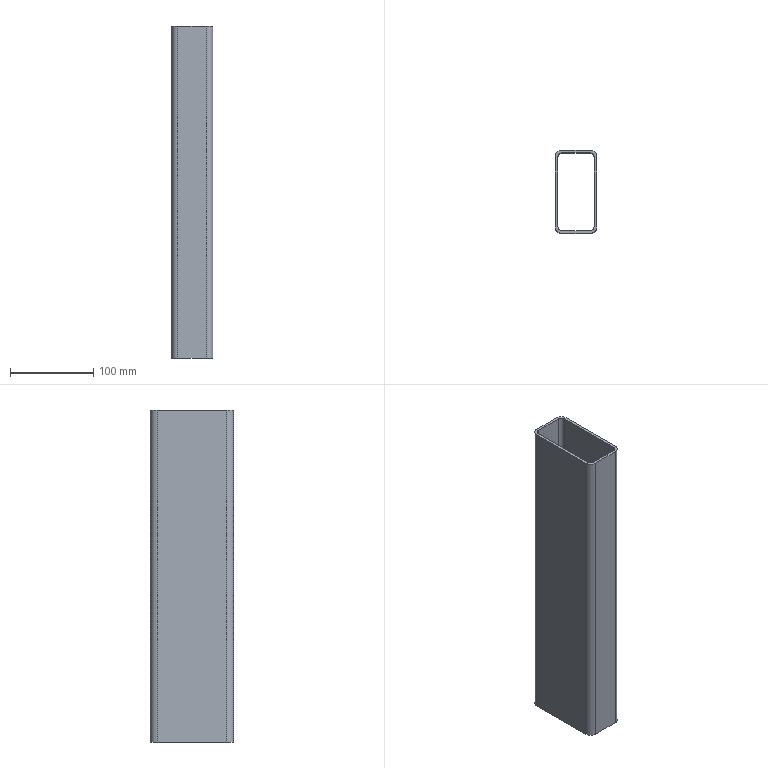Part | STEP file | KS D 3568 - 100 x 50 x 3.2 - 400 | 1 solid | 18 faces | box 50 x 100 x 400 mm | volume 353552 mm3 | plane 10 | cylinder 8 | commonest cylinder face diameters 9.6 x4 16 x4
STEP:
#1=CARTESIAN_POINT('',(0.,0.,0.));
#2=DIRECTION('',(0.,0.,1.));
#3=DIRECTION('',(1.,0.,0.));
#4=AXIS2_PLACEMENT_3D('',#1,#2,#3);
#5=CARTESIAN_POINT('',(17.,46.8,500.));
#6=VERTEX_POINT('',#5);
#7=CARTESIAN_POINT('',(-17.,46.8,500.));
#8=VERTEX_POINT('',#7);
#9=CARTESIAN_POINT('',(-8.5,46.8,500.));
#10=DIRECTION('',(-1.,0.,0.));
#11=VECTOR('',#10,1.);
#12=LINE('',#9,#11);
#13=CARTESIAN_POINT('',(0.,0.,500.));
#14=DIRECTION('',(0.,0.,1.));
#15=DIRECTION('',(1.,0.,0.));
#16=AXIS2_PLACEMENT_3D('',#13,#14,#15);
#17=PLANE('',#16);
#18=CARTESIAN_POINT('',(-8.5,46.8));
#19=DIRECTION('',(-1.,0.));
#20=VECTOR('',#19,1.);
#21=LINE('',#18,#20);
#22=(GEOMETRIC_REPRESENTATION_CONTEXT(2)PARAMETRIC_REPRESENTATION_CONTEXT()REPRESENTATION_CONTEXT('',''));
#23=DEFINITIONAL_REPRESENTATION('',(#21),#22);
#24=PCURVE('',#17,#23);
#25=CARTESIAN_POINT('',(-17.,46.8,0.));
#26=DIRECTION('',(0.,1.,0.));
#27=DIRECTION('',(1.,0.,0.));
#28=AXIS2_PLACEMENT_3D('',#25,#26,#27);
#29=PLANE('',#28);
#30=CARTESIAN_POINT('',(8.5,-500.));
#31=DIRECTION('',(-1.,0.));
#32=VECTOR('',#31,1.);
#33=LINE('',#30,#32);
#34=(GEOMETRIC_REPRESENTATION_CONTEXT(2)PARAMETRIC_REPRESENTATION_CONTEXT()REPRESENTATION_CONTEXT('',''));
#35=DEFINITIONAL_REPRESENTATION('',(#33),#34);
#36=PCURVE('',#29,#35);
#37=SURFACE_CURVE('',#12,(#24,#36),.PCURVE_S1.);
#38=EDGE_CURVE('',#6,#8,#37,.T.);
#39=ORIENTED_EDGE('',*,*,#38,.F.);
#40=CARTESIAN_POINT('',(21.8,42.,500.));
#41=VERTEX_POINT('',#40);
#42=CARTESIAN_POINT('',(17.,42.,500.));
#43=DIRECTION('',(0.,0.,1.));
#44=DIRECTION('',(-1.,0.,0.));
#45=AXIS2_PLACEMENT_3D('',#42,#43,#44);
#46=CIRCLE('',#45,4.8);
#47=CARTESIAN_POINT('',(17.,42.));
#48=DIRECTION('',(-1.,0.));
#49=AXIS2_PLACEMENT_2D('',#47,#48);
#50=CIRCLE('',#49,4.8);
#51=(GEOMETRIC_REPRESENTATION_CONTEXT(2)PARAMETRIC_REPRESENTATION_CONTEXT()REPRESENTATION_CONTEXT('',''));
#52=DEFINITIONAL_REPRESENTATION('',(#50),#51);
#53=PCURVE('',#17,#52);
#54=CARTESIAN_POINT('',(17.,42.,0.));
#55=DIRECTION('',(0.,0.,1.));
#56=DIRECTION('',(-1.,0.,0.));
#57=AXIS2_PLACEMENT_3D('',#54,#55,#56);
#58=CYLINDRICAL_SURFACE('',#57,4.8);
#59=CARTESIAN_POINT('',(0.,500.));
#60=DIRECTION('',(1.,0.));
#61=VECTOR('',#60,1.);
#62=LINE('',#59,#61);
#63=(GEOMETRIC_REPRESENTATION_CONTEXT(2)PARAMETRIC_REPRESENTATION_CONTEXT()REPRESENTATION_CONTEXT('',''));
#64=DEFINITIONAL_REPRESENTATION('',(#62),#63);
#65=PCURVE('',#58,#64);
#66=SURFACE_CURVE('',#46,(#53,#65),.PCURVE_S1.);
#67=EDGE_CURVE('',#41,#6,#66,.T.);
#68=ORIENTED_EDGE('',*,*,#67,.F.);
#69=CARTESIAN_POINT('',(21.8,-42.,500.));
#70=VERTEX_POINT('',#69);
#71=CARTESIAN_POINT('',(21.8,21.,500.));
#72=DIRECTION('',(0.,1.,0.));
#73=VECTOR('',#72,1.);
#74=LINE('',#71,#73);
#75=CARTESIAN_POINT('',(21.8,21.));
#76=DIRECTION('',(0.,1.));
#77=VECTOR('',#76,1.);
#78=LINE('',#75,#77);
#79=(GEOMETRIC_REPRESENTATION_CONTEXT(2)PARAMETRIC_REPRESENTATION_CONTEXT()REPRESENTATION_CONTEXT('',''));
#80=DEFINITIONAL_REPRESENTATION('',(#78),#79);
#81=PCURVE('',#17,#80);
#82=CARTESIAN_POINT('',(21.8,42.,0.));
#83=DIRECTION('',(1.,0.,0.));
#84=DIRECTION('',(0.,1.,0.));
#85=AXIS2_PLACEMENT_3D('',#82,#83,#84);
#86=PLANE('',#85);
#87=CARTESIAN_POINT('',(-21.,500.));
#88=DIRECTION('',(1.,0.));
#89=VECTOR('',#88,1.);
#90=LINE('',#87,#89);
#91=(GEOMETRIC_REPRESENTATION_CONTEXT(2)PARAMETRIC_REPRESENTATION_CONTEXT()REPRESENTATION_CONTEXT('',''));
#92=DEFINITIONAL_REPRESENTATION('',(#90),#91);
#93=PCURVE('',#86,#92);
#94=SURFACE_CURVE('',#74,(#81,#93),.PCURVE_S1.);
#95=EDGE_CURVE('',#70,#41,#94,.T.);
#96=ORIENTED_EDGE('',*,*,#95,.F.);
#97=CARTESIAN_POINT('',(17.,-46.8,500.));
#98=VERTEX_POINT('',#97);
#99=CARTESIAN_POINT('',(17.,-42.,500.));
#100=DIRECTION('',(0.,0.,1.));
#101=DIRECTION('',(0.,1.,0.));
#102=AXIS2_PLACEMENT_3D('',#99,#100,#101);
#103=CIRCLE('',#102,4.8);
#104=CARTESIAN_POINT('',(17.,-42.));
#105=DIRECTION('',(0.,1.));
#106=AXIS2_PLACEMENT_2D('',#104,#105);
#107=CIRCLE('',#106,4.8);
#108=(GEOMETRIC_REPRESENTATION_CONTEXT(2)PARAMETRIC_REPRESENTATION_CONTEXT()REPRESENTATION_CONTEXT('',''));
#109=DEFINITIONAL_REPRESENTATION('',(#107),#108);
#110=PCURVE('',#17,#109);
#111=CARTESIAN_POINT('',(17.,-42.,0.));
#112=DIRECTION('',(0.,0.,1.));
#113=DIRECTION('',(0.,1.,0.));
#114=AXIS2_PLACEMENT_3D('',#111,#112,#113);
#115=CYLINDRICAL_SURFACE('',#114,4.8);
#116=CARTESIAN_POINT('',(0.,500.));
#117=DIRECTION('',(1.,0.));
#118=VECTOR('',#117,1.);
#119=LINE('',#116,#118);
#120=(GEOMETRIC_REPRESENTATION_CONTEXT(2)PARAMETRIC_REPRESENTATION_CONTEXT()REPRESENTATION_CONTEXT('',''));
#121=DEFINITIONAL_REPRESENTATION('',(#119),#120);
#122=PCURVE('',#115,#121);
#123=SURFACE_CURVE('',#103,(#110,#122),.PCURVE_S1.);
#124=EDGE_CURVE('',#98,#70,#123,.T.);
#125=ORIENTED_EDGE('',*,*,#124,.F.);
#126=CARTESIAN_POINT('',(-17.,-46.8,500.));
#127=VERTEX_POINT('',#126);
#128=CARTESIAN_POINT('',(8.5,-46.8,500.));
#129=DIRECTION('',(1.,0.,0.));
#130=VECTOR('',#129,1.);
#131=LINE('',#128,#130);
#132=CARTESIAN_POINT('',(8.5,-46.8));
#133=DIRECTION('',(1.,0.));
#134=VECTOR('',#133,1.);
#135=LINE('',#132,#134);
#136=(GEOMETRIC_REPRESENTATION_CONTEXT(2)PARAMETRIC_REPRESENTATION_CONTEXT()REPRESENTATION_CONTEXT('',''));
#137=DEFINITIONAL_REPRESENTATION('',(#135),#136);
#138=PCURVE('',#17,#137);
#139=CARTESIAN_POINT('',(17.,-46.8,0.));
#140=DIRECTION('',(0.,-1.,0.));
#141=DIRECTION('',(0.,0.,-1.));
#142=AXIS2_PLACEMENT_3D('',#139,#140,#141);
#143=PLANE('',#142);
#144=CARTESIAN_POINT('',(-500.,-8.5));
#145=DIRECTION('',(0.,1.));
#146=VECTOR('',#145,1.);
#147=LINE('',#144,#146);
#148=(GEOMETRIC_REPRESENTATION_CONTEXT(2)PARAMETRIC_REPRESENTATION_CONTEXT()REPRESENTATION_CONTEXT('',''));
#149=DEFINITIONAL_REPRESENTATION('',(#147),#148);
#150=PCURVE('',#143,#149);
#151=SURFACE_CURVE('',#131,(#138,#150),.PCURVE_S1.);
#152=EDGE_CURVE('',#127,#98,#151,.T.);
#153=ORIENTED_EDGE('',*,*,#152,.F.);
#154=CARTESIAN_POINT('',(-21.8,-42.,500.));
#155=VERTEX_POINT('',#154);
#156=CARTESIAN_POINT('',(-17.,-42.,500.));
#157=DIRECTION('',(0.,0.,1.));
#158=DIRECTION('',(1.,0.,0.));
#159=AXIS2_PLACEMENT_3D('',#156,#157,#158);
#160=CIRCLE('',#159,4.8);
#161=CARTESIAN_POINT('',(-17.,-42.));
#162=DIRECTION('',(1.,0.));
#163=AXIS2_PLACEMENT_2D('',#161,#162);
#164=CIRCLE('',#163,4.8);
#165=(GEOMETRIC_REPRESENTATION_CONTEXT(2)PARAMETRIC_REPRESENTATION_CONTEXT()REPRESENTATION_CONTEXT('',''));
#166=DEFINITIONAL_REPRESENTATION('',(#164),#165);
#167=PCURVE('',#17,#166);
#168=CARTESIAN_POINT('',(-17.,-42.,0.));
#169=DIRECTION('',(0.,0.,1.));
#170=DIRECTION('',(1.,0.,0.));
#171=AXIS2_PLACEMENT_3D('',#168,#169,#170);
#172=CYLINDRICAL_SURFACE('',#171,4.8);
#173=CARTESIAN_POINT('',(0.,500.));
#174=DIRECTION('',(1.,0.));
#175=VECTOR('',#174,1.);
#176=LINE('',#173,#175);
#177=(GEOMETRIC_REPRESENTATION_CONTEXT(2)PARAMETRIC_REPRESENTATION_CONTEXT()REPRESENTATION_CONTEXT('',''));
#178=DEFINITIONAL_REPRESENTATION('',(#176),#177);
#179=PCURVE('',#172,#178);
#180=SURFACE_CURVE('',#160,(#167,#179),.PCURVE_S1.);
#181=EDGE_CURVE('',#155,#127,#180,.T.);
#182=ORIENTED_EDGE('',*,*,#181,.F.);
#183=CARTESIAN_POINT('',(-21.8,42.,500.));
#184=VERTEX_POINT('',#183);
#185=CARTESIAN_POINT('',(-21.8,-21.,500.));
#186=DIRECTION('',(0.,-1.,0.));
#187=VECTOR('',#186,1.);
#188=LINE('',#185,#187);
#189=CARTESIAN_POINT('',(-21.8,-21.));
#190=DIRECTION('',(0.,-1.));
#191=VECTOR('',#190,1.);
#192=LINE('',#189,#191);
#193=(GEOMETRIC_REPRESENTATION_CONTEXT(2)PARAMETRIC_REPRESENTATION_CONTEXT()REPRESENTATION_CONTEXT('',''));
#194=DEFINITIONAL_REPRESENTATION('',(#192),#193);
#195=PCURVE('',#17,#194);
#196=CARTESIAN_POINT('',(-21.8,-42.,0.));
#197=DIRECTION('',(-1.,0.,0.));
#198=DIRECTION('',(0.,1.,0.));
#199=AXIS2_PLACEMENT_3D('',#196,#197,#198);
#200=PLANE('',#199);
#201=CARTESIAN_POINT('',(21.,-500.));
#202=DIRECTION('',(-1.,0.));
#203=VECTOR('',#202,1.);
#204=LINE('',#201,#203);
#205=(GEOMETRIC_REPRESENTATION_CONTEXT(2)PARAMETRIC_REPRESENTATION_CONTEXT()REPRESENTATION_CONTEXT('',''));
#206=DEFINITIONAL_REPRESENTATION('',(#204),#205);
#207=PCURVE('',#200,#206);
#208=SURFACE_CURVE('',#188,(#195,#207),.PCURVE_S1.);
#209=EDGE_CURVE('',#184,#155,#208,.T.);
#210=ORIENTED_EDGE('',*,*,#209,.F.);
#211=CARTESIAN_POINT('',(-17.,42.,500.));
#212=DIRECTION('',(0.,0.,1.));
#213=DIRECTION('',(0.,-1.,0.));
#214=AXIS2_PLACEMENT_3D('',#211,#212,#213);
#215=CIRCLE('',#214,4.8);
#216=CARTESIAN_POINT('',(-17.,42.));
#217=DIRECTION('',(0.,-1.));
#218=AXIS2_PLACEMENT_2D('',#216,#217);
#219=CIRCLE('',#218,4.8);
#220=(GEOMETRIC_REPRESENTATION_CONTEXT(2)PARAMETRIC_REPRESENTATION_CONTEXT()REPRESENTATION_CONTEXT('',''));
#221=DEFINITIONAL_REPRESENTATION('',(#219),#220);
#222=PCURVE('',#17,#221);
#223=CARTESIAN_POINT('',(-17.,42.,0.));
#224=DIRECTION('',(0.,0.,1.));
#225=DIRECTION('',(0.,-1.,0.));
#226=AXIS2_PLACEMENT_3D('',#223,#224,#225);
#227=CYLINDRICAL_SURFACE('',#226,4.8);
#228=CARTESIAN_POINT('',(0.,500.));
#229=DIRECTION('',(1.,0.));
#230=VECTOR('',#229,1.);
#231=LINE('',#228,#230);
#232=(GEOMETRIC_REPRESENTATION_CONTEXT(2)PARAMETRIC_REPRESENTATION_CONTEXT()REPRESENTATION_CONTEXT('',''));
#233=DEFINITIONAL_REPRESENTATION('',(#231),#232);
#234=PCURVE('',#227,#233);
#235=SURFACE_CURVE('',#215,(#222,#234),.PCURVE_S1.);
#236=EDGE_CURVE('',#8,#184,#235,.T.);
#237=ORIENTED_EDGE('',*,*,#236,.F.);
#238=EDGE_LOOP('',(#39,#68,#96,#125,#153,#182,#210,#237));
#239=FACE_BOUND('',#238,.T.);
#240=CARTESIAN_POINT('',(-25.,-42.,500.));
#241=VERTEX_POINT('',#240);
#242=CARTESIAN_POINT('',(-25.,42.,500.));
#243=VERTEX_POINT('',#242);
#244=CARTESIAN_POINT('',(-25.,-21.,500.));
#245=DIRECTION('',(0.,1.,0.));
#246=VECTOR('',#245,1.);
#247=LINE('',#244,#246);
#248=CARTESIAN_POINT('',(-25.,-21.));
#249=DIRECTION('',(0.,1.));
#250=VECTOR('',#249,1.);
#251=LINE('',#248,#250);
#252=(GEOMETRIC_REPRESENTATION_CONTEXT(2)PARAMETRIC_REPRESENTATION_CONTEXT()REPRESENTATION_CONTEXT('',''));
#253=DEFINITIONAL_REPRESENTATION('',(#251),#252);
#254=PCURVE('',#17,#253);
#255=CARTESIAN_POINT('',(-25.,-42.,0.));
#256=DIRECTION('',(-1.,0.,0.));
#257=DIRECTION('',(0.,1.,0.));
#258=AXIS2_PLACEMENT_3D('',#255,#256,#257);
#259=PLANE('',#258);
#260=CARTESIAN_POINT('',(21.,-500.));
#261=DIRECTION('',(1.,0.));
#262=VECTOR('',#261,1.);
#263=LINE('',#260,#262);
#264=(GEOMETRIC_REPRESENTATION_CONTEXT(2)PARAMETRIC_REPRESENTATION_CONTEXT()REPRESENTATION_CONTEXT('',''));
#265=DEFINITIONAL_REPRESENTATION('',(#263),#264);
#266=PCURVE('',#259,#265);
#267=SURFACE_CURVE('',#247,(#254,#266),.PCURVE_S1.);
#268=EDGE_CURVE('',#241,#243,#267,.T.);
#269=ORIENTED_EDGE('',*,*,#268,.F.);
#270=CARTESIAN_POINT('',(-17.,-50.,500.));
#271=VERTEX_POINT('',#270);
#272=CARTESIAN_POINT('',(-17.,-42.,500.));
#273=DIRECTION('',(0.,0.,-1.));
#274=DIRECTION('',(1.,0.,0.));
#275=AXIS2_PLACEMENT_3D('',#272,#273,#274);
#276=CIRCLE('',#275,8.);
#277=CARTESIAN_POINT('',(-9.,-42.));
#278=CARTESIAN_POINT('',(-9.,-55.856));
#279=CARTESIAN_POINT('',(-21.,-48.928));
#280=CARTESIAN_POINT('',(-33.,-42.));
#281=CARTESIAN_POINT('',(-21.,-35.072));
#282=CARTESIAN_POINT('',(-9.,-28.144));
#283=CARTESIAN_POINT('',(-9.,-42.));
#284=(BOUNDED_CURVE()B_SPLINE_CURVE(2,(#277,#278,#279,#280,#281,#282,#283),.UNSPECIFIED.,.T.,.F.)B_SPLINE_CURVE_WITH_KNOTS((1,2,2,2,2,1),(-2.094,0.,2.094,4.189,6.283,8.378),.UNSPECIFIED.)CURVE()GEOMETRIC_REPRESENTATION_ITEM()RATIONAL_B_SPLINE_CURVE((1.,0.5,1.,0.5,1.,0.5,1.))REPRESENTATION_ITEM(''));
#285=(GEOMETRIC_REPRESENTATION_CONTEXT(2)PARAMETRIC_REPRESENTATION_CONTEXT()REPRESENTATION_CONTEXT('',''));
#286=DEFINITIONAL_REPRESENTATION('',(#284),#285);
#287=PCURVE('',#17,#286);
#288=CARTESIAN_POINT('',(-17.,-42.,0.));
#289=DIRECTION('',(0.,0.,1.));
#290=DIRECTION('',(1.,0.,0.));
#291=AXIS2_PLACEMENT_3D('',#288,#289,#290);
#292=CYLINDRICAL_SURFACE('',#291,8.);
#293=CARTESIAN_POINT('',(6.283,500.));
#294=DIRECTION('',(-1.,0.));
#295=VECTOR('',#294,1.);
#296=LINE('',#293,#295);
#297=(GEOMETRIC_REPRESENTATION_CONTEXT(2)PARAMETRIC_REPRESENTATION_CONTEXT()REPRESENTATION_CONTEXT('',''));
#298=DEFINITIONAL_REPRESENTATION('',(#296),#297);
#299=PCURVE('',#292,#298);
#300=SURFACE_CURVE('',#276,(#287,#299),.PCURVE_S1.);
#301=EDGE_CURVE('',#271,#241,#300,.T.);
#302=ORIENTED_EDGE('',*,*,#301,.F.);
#303=CARTESIAN_POINT('',(17.,-50.,500.));
#304=VERTEX_POINT('',#303);
#305=CARTESIAN_POINT('',(8.5,-50.,500.));
#306=DIRECTION('',(-1.,0.,0.));
#307=VECTOR('',#306,1.);
#308=LINE('',#305,#307);
#309=CARTESIAN_POINT('',(8.5,-50.));
#310=DIRECTION('',(-1.,0.));
#311=VECTOR('',#310,1.);
#312=LINE('',#309,#311);
#313=(GEOMETRIC_REPRESENTATION_CONTEXT(2)PARAMETRIC_REPRESENTATION_CONTEXT()REPRESENTATION_CONTEXT('',''));
#314=DEFINITIONAL_REPRESENTATION('',(#312),#313);
#315=PCURVE('',#17,#314);
#316=CARTESIAN_POINT('',(17.,-50.,0.));
#317=DIRECTION('',(0.,-1.,0.));
#318=DIRECTION('',(-1.,0.,0.));
#319=AXIS2_PLACEMENT_3D('',#316,#317,#318);
#320=PLANE('',#319);
#321=CARTESIAN_POINT('',(8.5,-500.));
#322=DIRECTION('',(1.,0.));
#323=VECTOR('',#322,1.);
#324=LINE('',#321,#323);
#325=(GEOMETRIC_REPRESENTATION_CONTEXT(2)PARAMETRIC_REPRESENTATION_CONTEXT()REPRESENTATION_CONTEXT('',''));
#326=DEFINITIONAL_REPRESENTATION('',(#324),#325);
#327=PCURVE('',#320,#326);
#328=SURFACE_CURVE('',#308,(#315,#327),.PCURVE_S1.);
#329=EDGE_CURVE('',#304,#271,#328,.T.);
#330=ORIENTED_EDGE('',*,*,#329,.F.);
#331=CARTESIAN_POINT('',(25.,-42.,500.));
#332=VERTEX_POINT('',#331);
#333=CARTESIAN_POINT('',(17.,-42.,500.));
#334=DIRECTION('',(0.,0.,-1.));
#335=DIRECTION('',(0.,1.,0.));
#336=AXIS2_PLACEMENT_3D('',#333,#334,#335);
#337=CIRCLE('',#336,8.);
#338=CARTESIAN_POINT('',(17.,-34.));
#339=CARTESIAN_POINT('',(30.856,-34.));
#340=CARTESIAN_POINT('',(23.928,-46.));
#341=CARTESIAN_POINT('',(17.,-58.));
#342=CARTESIAN_POINT('',(10.072,-46.));
#343=CARTESIAN_POINT('',(3.144,-34.));
#344=CARTESIAN_POINT('',(17.,-34.));
#345=(BOUNDED_CURVE()B_SPLINE_CURVE(2,(#338,#339,#340,#341,#342,#343,#344),.UNSPECIFIED.,.T.,.F.)B_SPLINE_CURVE_WITH_KNOTS((1,2,2,2,2,1),(-2.094,0.,2.094,4.189,6.283,8.378),.UNSPECIFIED.)CURVE()GEOMETRIC_REPRESENTATION_ITEM()RATIONAL_B_SPLINE_CURVE((1.,0.5,1.,0.5,1.,0.5,1.))REPRESENTATION_ITEM(''));
#346=(GEOMETRIC_REPRESENTATION_CONTEXT(2)PARAMETRIC_REPRESENTATION_CONTEXT()REPRESENTATION_CONTEXT('',''));
#347=DEFINITIONAL_REPRESENTATION('',(#345),#346);
#348=PCURVE('',#17,#347);
#349=CARTESIAN_POINT('',(17.,-42.,0.));
#350=DIRECTION('',(0.,0.,1.));
#351=DIRECTION('',(0.,1.,0.));
#352=AXIS2_PLACEMENT_3D('',#349,#350,#351);
#353=CYLINDRICAL_SURFACE('',#352,8.);
#354=CARTESIAN_POINT('',(6.283,500.));
#355=DIRECTION('',(-1.,0.));
#356=VECTOR('',#355,1.);
#357=LINE('',#354,#356);
#358=(GEOMETRIC_REPRESENTATION_CONTEXT(2)PARAMETRIC_REPRESENTATION_CONTEXT()REPRESENTATION_CONTEXT('',''));
#359=DEFINITIONAL_REPRESENTATION('',(#357),#358);
#360=PCURVE('',#353,#359);
#361=SURFACE_CURVE('',#337,(#348,#360),.PCURVE_S1.);
#362=EDGE_CURVE('',#332,#304,#361,.T.);
#363=ORIENTED_EDGE('',*,*,#362,.F.);
#364=CARTESIAN_POINT('',(25.,42.,500.));
#365=VERTEX_POINT('',#364);
#366=CARTESIAN_POINT('',(25.,21.,500.));
#367=DIRECTION('',(0.,-1.,0.));
#368=VECTOR('',#367,1.);
#369=LINE('',#366,#368);
#370=CARTESIAN_POINT('',(25.,21.));
#371=DIRECTION('',(0.,-1.));
#372=VECTOR('',#371,1.);
#373=LINE('',#370,#372);
#374=(GEOMETRIC_REPRESENTATION_CONTEXT(2)PARAMETRIC_REPRESENTATION_CONTEXT()REPRESENTATION_CONTEXT('',''));
#375=DEFINITIONAL_REPRESENTATION('',(#373),#374);
#376=PCURVE('',#17,#375);
#377=CARTESIAN_POINT('',(25.,42.,0.));
#378=DIRECTION('',(1.,0.,0.));
#379=DIRECTION('',(0.,-1.,0.));
#380=AXIS2_PLACEMENT_3D('',#377,#378,#379);
#381=PLANE('',#380);
#382=CARTESIAN_POINT('',(21.,-500.));
#383=DIRECTION('',(1.,0.));
#384=VECTOR('',#383,1.);
#385=LINE('',#382,#384);
#386=(GEOMETRIC_REPRESENTATION_CONTEXT(2)PARAMETRIC_REPRESENTATION_CONTEXT()REPRESENTATION_CONTEXT('',''));
#387=DEFINITIONAL_REPRESENTATION('',(#385),#386);
#388=PCURVE('',#381,#387);
#389=SURFACE_CURVE('',#369,(#376,#388),.PCURVE_S1.);
#390=EDGE_CURVE('',#365,#332,#389,.T.);
#391=ORIENTED_EDGE('',*,*,#390,.F.);
#392=CARTESIAN_POINT('',(17.,50.,500.));
#393=VERTEX_POINT('',#392);
#394=CARTESIAN_POINT('',(17.,42.,500.));
#395=DIRECTION('',(0.,0.,-1.));
#396=DIRECTION('',(-1.,0.,0.));
#397=AXIS2_PLACEMENT_3D('',#394,#395,#396);
#398=CIRCLE('',#397,8.);
#399=CARTESIAN_POINT('',(9.,42.));
#400=CARTESIAN_POINT('',(9.,55.856));
#401=CARTESIAN_POINT('',(21.,48.928));
#402=CARTESIAN_POINT('',(33.,42.));
#403=CARTESIAN_POINT('',(21.,35.072));
#404=CARTESIAN_POINT('',(9.,28.144));
#405=CARTESIAN_POINT('',(9.,42.));
#406=(BOUNDED_CURVE()B_SPLINE_CURVE(2,(#399,#400,#401,#402,#403,#404,#405),.UNSPECIFIED.,.T.,.F.)B_SPLINE_CURVE_WITH_KNOTS((1,2,2,2,2,1),(-2.094,0.,2.094,4.189,6.283,8.378),.UNSPECIFIED.)CURVE()GEOMETRIC_REPRESENTATION_ITEM()RATIONAL_B_SPLINE_CURVE((1.,0.5,1.,0.5,1.,0.5,1.))REPRESENTATION_ITEM(''));
#407=(GEOMETRIC_REPRESENTATION_CONTEXT(2)PARAMETRIC_REPRESENTATION_CONTEXT()REPRESENTATION_CONTEXT('',''));
#408=DEFINITIONAL_REPRESENTATION('',(#406),#407);
#409=PCURVE('',#17,#408);
#410=CARTESIAN_POINT('',(17.,42.,0.));
#411=DIRECTION('',(0.,0.,1.));
#412=DIRECTION('',(-1.,0.,0.));
#413=AXIS2_PLACEMENT_3D('',#410,#411,#412);
#414=CYLINDRICAL_SURFACE('',#413,8.);
#415=CARTESIAN_POINT('',(6.283,500.));
#416=DIRECTION('',(-1.,0.));
#417=VECTOR('',#416,1.);
#418=LINE('',#415,#417);
#419=(GEOMETRIC_REPRESENTATION_CONTEXT(2)PARAMETRIC_REPRESENTATION_CONTEXT()REPRESENTATION_CONTEXT('',''));
#420=DEFINITIONAL_REPRESENTATION('',(#418),#419);
#421=PCURVE('',#414,#420);
#422=SURFACE_CURVE('',#398,(#409,#421),.PCURVE_S1.);
#423=EDGE_CURVE('',#393,#365,#422,.T.);
#424=ORIENTED_EDGE('',*,*,#423,.F.);
#425=CARTESIAN_POINT('',(-17.,50.,500.));
#426=VERTEX_POINT('',#425);
#427=CARTESIAN_POINT('',(-8.5,50.,500.));
#428=DIRECTION('',(1.,0.,0.));
#429=VECTOR('',#428,1.);
#430=LINE('',#427,#429);
#431=CARTESIAN_POINT('',(-8.5,50.));
#432=DIRECTION('',(1.,0.));
#433=VECTOR('',#432,1.);
#434=LINE('',#431,#433);
#435=(GEOMETRIC_REPRESENTATION_CONTEXT(2)PARAMETRIC_REPRESENTATION_CONTEXT()REPRESENTATION_CONTEXT('',''));
#436=DEFINITIONAL_REPRESENTATION('',(#434),#435);
#437=PCURVE('',#17,#436);
#438=CARTESIAN_POINT('',(-17.,50.,0.));
#439=DIRECTION('',(0.,1.,0.));
#440=DIRECTION('',(1.,0.,0.));
#441=AXIS2_PLACEMENT_3D('',#438,#439,#440);
#442=PLANE('',#441);
#443=CARTESIAN_POINT('',(8.5,-500.));
#444=DIRECTION('',(1.,0.));
#445=VECTOR('',#444,1.);
#446=LINE('',#443,#445);
#447=(GEOMETRIC_REPRESENTATION_CONTEXT(2)PARAMETRIC_REPRESENTATION_CONTEXT()REPRESENTATION_CONTEXT('',''));
#448=DEFINITIONAL_REPRESENTATION('',(#446),#447);
#449=PCURVE('',#442,#448);
#450=SURFACE_CURVE('',#430,(#437,#449),.PCURVE_S1.);
#451=EDGE_CURVE('',#426,#393,#450,.T.);
#452=ORIENTED_EDGE('',*,*,#451,.F.);
#453=CARTESIAN_POINT('',(-17.,42.,500.));
#454=DIRECTION('',(0.,0.,-1.));
#455=DIRECTION('',(0.,-1.,0.));
#456=AXIS2_PLACEMENT_3D('',#453,#454,#455);
#457=CIRCLE('',#456,8.);
#458=CARTESIAN_POINT('',(-17.,34.));
#459=CARTESIAN_POINT('',(-30.856,34.));
#460=CARTESIAN_POINT('',(-23.928,46.));
#461=CARTESIAN_POINT('',(-17.,58.));
#462=CARTESIAN_POINT('',(-10.072,46.));
#463=CARTESIAN_POINT('',(-3.144,34.));
#464=CARTESIAN_POINT('',(-17.,34.));
#465=(BOUNDED_CURVE()B_SPLINE_CURVE(2,(#458,#459,#460,#461,#462,#463,#464),.UNSPECIFIED.,.T.,.F.)B_SPLINE_CURVE_WITH_KNOTS((1,2,2,2,2,1),(-2.094,0.,2.094,4.189,6.283,8.378),.UNSPECIFIED.)CURVE()GEOMETRIC_REPRESENTATION_ITEM()RATIONAL_B_SPLINE_CURVE((1.,0.5,1.,0.5,1.,0.5,1.))REPRESENTATION_ITEM(''));
#466=(GEOMETRIC_REPRESENTATION_CONTEXT(2)PARAMETRIC_REPRESENTATION_CONTEXT()REPRESENTATION_CONTEXT('',''));
#467=DEFINITIONAL_REPRESENTATION('',(#465),#466);
#468=PCURVE('',#17,#467);
#469=CARTESIAN_POINT('',(-17.,42.,0.));
#470=DIRECTION('',(0.,0.,1.));
#471=DIRECTION('',(0.,-1.,0.));
#472=AXIS2_PLACEMENT_3D('',#469,#470,#471);
#473=CYLINDRICAL_SURFACE('',#472,8.);
#474=CARTESIAN_POINT('',(6.283,500.));
#475=DIRECTION('',(-1.,0.));
#476=VECTOR('',#475,1.);
#477=LINE('',#474,#476);
#478=(GEOMETRIC_REPRESENTATION_CONTEXT(2)PARAMETRIC_REPRESENTATION_CONTEXT()REPRESENTATION_CONTEXT('',''));
#479=DEFINITIONAL_REPRESENTATION('',(#477),#478);
#480=PCURVE('',#473,#479);
#481=SURFACE_CURVE('',#457,(#468,#480),.PCURVE_S1.);
#482=EDGE_CURVE('',#243,#426,#481,.T.);
#483=ORIENTED_EDGE('',*,*,#482,.F.);
#484=EDGE_LOOP('',(#269,#302,#330,#363,#391,#424,#452,#483));
#485=FACE_BOUND('',#484,.T.);
#486=ADVANCED_FACE('',(#239,#485),#17,.T.);
#487=CARTESIAN_POINT('',(17.,46.8,100.));
#488=VERTEX_POINT('',#487);
#489=CARTESIAN_POINT('',(-17.,46.8,100.));
#490=VERTEX_POINT('',#489);
#491=CARTESIAN_POINT('',(-8.5,46.8,100.));
#492=DIRECTION('',(-1.,0.,0.));
#493=VECTOR('',#492,1.);
#494=LINE('',#491,#493);
#495=CARTESIAN_POINT('',(0.,0.,100.));
#496=DIRECTION('',(0.,0.,1.));
#497=DIRECTION('',(1.,0.,0.));
#498=AXIS2_PLACEMENT_3D('',#495,#496,#497);
#499=PLANE('',#498);
#500=CARTESIAN_POINT('',(-8.5,46.8));
#501=DIRECTION('',(-1.,0.));
#502=VECTOR('',#501,1.);
#503=LINE('',#500,#502);
#504=(GEOMETRIC_REPRESENTATION_CONTEXT(2)PARAMETRIC_REPRESENTATION_CONTEXT()REPRESENTATION_CONTEXT('',''));
#505=DEFINITIONAL_REPRESENTATION('',(#503),#504);
#506=PCURVE('',#499,#505);
#507=CARTESIAN_POINT('',(8.5,-100.));
#508=DIRECTION('',(-1.,0.));
#509=VECTOR('',#508,1.);
#510=LINE('',#507,#509);
#511=(GEOMETRIC_REPRESENTATION_CONTEXT(2)PARAMETRIC_REPRESENTATION_CONTEXT()REPRESENTATION_CONTEXT('',''));
#512=DEFINITIONAL_REPRESENTATION('',(#510),#511);
#513=PCURVE('',#29,#512);
#514=SURFACE_CURVE('',#494,(#506,#513),.PCURVE_S1.);
#515=EDGE_CURVE('',#488,#490,#514,.T.);
#516=ORIENTED_EDGE('',*,*,#515,.T.);
#517=CARTESIAN_POINT('',(-21.8,42.,100.));
#518=VERTEX_POINT('',#517);
#519=CARTESIAN_POINT('',(-17.,42.,100.));
#520=DIRECTION('',(0.,0.,1.));
#521=DIRECTION('',(0.,-1.,0.));
#522=AXIS2_PLACEMENT_3D('',#519,#520,#521);
#523=CIRCLE('',#522,4.8);
#524=CARTESIAN_POINT('',(-17.,42.));
#525=DIRECTION('',(0.,-1.));
#526=AXIS2_PLACEMENT_2D('',#524,#525);
#527=CIRCLE('',#526,4.8);
#528=(GEOMETRIC_REPRESENTATION_CONTEXT(2)PARAMETRIC_REPRESENTATION_CONTEXT()REPRESENTATION_CONTEXT('',''));
#529=DEFINITIONAL_REPRESENTATION('',(#527),#528);
#530=PCURVE('',#499,#529);
#531=CARTESIAN_POINT('',(0.,100.));
#532=DIRECTION('',(1.,0.));
#533=VECTOR('',#532,1.);
#534=LINE('',#531,#533);
#535=(GEOMETRIC_REPRESENTATION_CONTEXT(2)PARAMETRIC_REPRESENTATION_CONTEXT()REPRESENTATION_CONTEXT('',''));
#536=DEFINITIONAL_REPRESENTATION('',(#534),#535);
#537=PCURVE('',#227,#536);
#538=SURFACE_CURVE('',#523,(#530,#537),.PCURVE_S1.);
#539=EDGE_CURVE('',#490,#518,#538,.T.);
#540=ORIENTED_EDGE('',*,*,#539,.T.);
#541=CARTESIAN_POINT('',(-21.8,-42.,100.));
#542=VERTEX_POINT('',#541);
#543=CARTESIAN_POINT('',(-21.8,-21.,100.));
#544=DIRECTION('',(0.,-1.,0.));
#545=VECTOR('',#544,1.);
#546=LINE('',#543,#545);
#547=CARTESIAN_POINT('',(-21.8,-21.));
#548=DIRECTION('',(0.,-1.));
#549=VECTOR('',#548,1.);
#550=LINE('',#547,#549);
#551=(GEOMETRIC_REPRESENTATION_CONTEXT(2)PARAMETRIC_REPRESENTATION_CONTEXT()REPRESENTATION_CONTEXT('',''));
#552=DEFINITIONAL_REPRESENTATION('',(#550),#551);
#553=PCURVE('',#499,#552);
#554=CARTESIAN_POINT('',(21.,-100.));
#555=DIRECTION('',(-1.,0.));
#556=VECTOR('',#555,1.);
#557=LINE('',#554,#556);
#558=(GEOMETRIC_REPRESENTATION_CONTEXT(2)PARAMETRIC_REPRESENTATION_CONTEXT()REPRESENTATION_CONTEXT('',''));
#559=DEFINITIONAL_REPRESENTATION('',(#557),#558);
#560=PCURVE('',#200,#559);
#561=SURFACE_CURVE('',#546,(#553,#560),.PCURVE_S1.);
#562=EDGE_CURVE('',#518,#542,#561,.T.);
#563=ORIENTED_EDGE('',*,*,#562,.T.);
#564=CARTESIAN_POINT('',(-17.,-46.8,100.));
#565=VERTEX_POINT('',#564);
#566=CARTESIAN_POINT('',(-17.,-42.,100.));
#567=DIRECTION('',(0.,0.,1.));
#568=DIRECTION('',(1.,0.,0.));
#569=AXIS2_PLACEMENT_3D('',#566,#567,#568);
#570=CIRCLE('',#569,4.8);
#571=CARTESIAN_POINT('',(-17.,-42.));
#572=DIRECTION('',(1.,0.));
#573=AXIS2_PLACEMENT_2D('',#571,#572);
#574=CIRCLE('',#573,4.8);
#575=(GEOMETRIC_REPRESENTATION_CONTEXT(2)PARAMETRIC_REPRESENTATION_CONTEXT()REPRESENTATION_CONTEXT('',''));
#576=DEFINITIONAL_REPRESENTATION('',(#574),#575);
#577=PCURVE('',#499,#576);
#578=CARTESIAN_POINT('',(0.,100.));
#579=DIRECTION('',(1.,0.));
#580=VECTOR('',#579,1.);
#581=LINE('',#578,#580);
#582=(GEOMETRIC_REPRESENTATION_CONTEXT(2)PARAMETRIC_REPRESENTATION_CONTEXT()REPRESENTATION_CONTEXT('',''));
#583=DEFINITIONAL_REPRESENTATION('',(#581),#582);
#584=PCURVE('',#172,#583);
#585=SURFACE_CURVE('',#570,(#577,#584),.PCURVE_S1.);
#586=EDGE_CURVE('',#542,#565,#585,.T.);
#587=ORIENTED_EDGE('',*,*,#586,.T.);
#588=CARTESIAN_POINT('',(17.,-46.8,100.));
#589=VERTEX_POINT('',#588);
#590=CARTESIAN_POINT('',(8.5,-46.8,100.));
#591=DIRECTION('',(1.,0.,0.));
#592=VECTOR('',#591,1.);
#593=LINE('',#590,#592);
#594=CARTESIAN_POINT('',(8.5,-46.8));
#595=DIRECTION('',(1.,0.));
#596=VECTOR('',#595,1.);
#597=LINE('',#594,#596);
#598=(GEOMETRIC_REPRESENTATION_CONTEXT(2)PARAMETRIC_REPRESENTATION_CONTEXT()REPRESENTATION_CONTEXT('',''));
#599=DEFINITIONAL_REPRESENTATION('',(#597),#598);
#600=PCURVE('',#499,#599);
#601=CARTESIAN_POINT('',(-100.,-8.5));
#602=DIRECTION('',(0.,1.));
#603=VECTOR('',#602,1.);
#604=LINE('',#601,#603);
#605=(GEOMETRIC_REPRESENTATION_CONTEXT(2)PARAMETRIC_REPRESENTATION_CONTEXT()REPRESENTATION_CONTEXT('',''));
#606=DEFINITIONAL_REPRESENTATION('',(#604),#605);
#607=PCURVE('',#143,#606);
#608=SURFACE_CURVE('',#593,(#600,#607),.PCURVE_S1.);
#609=EDGE_CURVE('',#565,#589,#608,.T.);
#610=ORIENTED_EDGE('',*,*,#609,.T.);
#611=CARTESIAN_POINT('',(21.8,-42.,100.));
#612=VERTEX_POINT('',#611);
#613=CARTESIAN_POINT('',(17.,-42.,100.));
#614=DIRECTION('',(0.,0.,1.));
#615=DIRECTION('',(0.,1.,0.));
#616=AXIS2_PLACEMENT_3D('',#613,#614,#615);
#617=CIRCLE('',#616,4.8);
#618=CARTESIAN_POINT('',(17.,-42.));
#619=DIRECTION('',(0.,1.));
#620=AXIS2_PLACEMENT_2D('',#618,#619);
#621=CIRCLE('',#620,4.8);
#622=(GEOMETRIC_REPRESENTATION_CONTEXT(2)PARAMETRIC_REPRESENTATION_CONTEXT()REPRESENTATION_CONTEXT('',''));
#623=DEFINITIONAL_REPRESENTATION('',(#621),#622);
#624=PCURVE('',#499,#623);
#625=CARTESIAN_POINT('',(0.,100.));
#626=DIRECTION('',(1.,0.));
#627=VECTOR('',#626,1.);
#628=LINE('',#625,#627);
#629=(GEOMETRIC_REPRESENTATION_CONTEXT(2)PARAMETRIC_REPRESENTATION_CONTEXT()REPRESENTATION_CONTEXT('',''));
#630=DEFINITIONAL_REPRESENTATION('',(#628),#629);
#631=PCURVE('',#115,#630);
#632=SURFACE_CURVE('',#617,(#624,#631),.PCURVE_S1.);
#633=EDGE_CURVE('',#589,#612,#632,.T.);
#634=ORIENTED_EDGE('',*,*,#633,.T.);
#635=CARTESIAN_POINT('',(21.8,42.,100.));
#636=VERTEX_POINT('',#635);
#637=CARTESIAN_POINT('',(21.8,21.,100.));
#638=DIRECTION('',(0.,1.,0.));
#639=VECTOR('',#638,1.);
#640=LINE('',#637,#639);
#641=CARTESIAN_POINT('',(21.8,21.));
#642=DIRECTION('',(0.,1.));
#643=VECTOR('',#642,1.);
#644=LINE('',#641,#643);
#645=(GEOMETRIC_REPRESENTATION_CONTEXT(2)PARAMETRIC_REPRESENTATION_CONTEXT()REPRESENTATION_CONTEXT('',''));
#646=DEFINITIONAL_REPRESENTATION('',(#644),#645);
#647=PCURVE('',#499,#646);
#648=CARTESIAN_POINT('',(-21.,100.));
#649=DIRECTION('',(1.,0.));
#650=VECTOR('',#649,1.);
#651=LINE('',#648,#650);
#652=(GEOMETRIC_REPRESENTATION_CONTEXT(2)PARAMETRIC_REPRESENTATION_CONTEXT()REPRESENTATION_CONTEXT('',''));
#653=DEFINITIONAL_REPRESENTATION('',(#651),#652);
#654=PCURVE('',#86,#653);
#655=SURFACE_CURVE('',#640,(#647,#654),.PCURVE_S1.);
#656=EDGE_CURVE('',#612,#636,#655,.T.);
#657=ORIENTED_EDGE('',*,*,#656,.T.);
#658=CARTESIAN_POINT('',(17.,42.,100.));
#659=DIRECTION('',(0.,0.,1.));
#660=DIRECTION('',(-1.,0.,0.));
#661=AXIS2_PLACEMENT_3D('',#658,#659,#660);
#662=CIRCLE('',#661,4.8);
#663=CARTESIAN_POINT('',(17.,42.));
#664=DIRECTION('',(-1.,0.));
#665=AXIS2_PLACEMENT_2D('',#663,#664);
#666=CIRCLE('',#665,4.8);
#667=(GEOMETRIC_REPRESENTATION_CONTEXT(2)PARAMETRIC_REPRESENTATION_CONTEXT()REPRESENTATION_CONTEXT('',''));
#668=DEFINITIONAL_REPRESENTATION('',(#666),#667);
#669=PCURVE('',#499,#668);
#670=CARTESIAN_POINT('',(0.,100.));
#671=DIRECTION('',(1.,0.));
#672=VECTOR('',#671,1.);
#673=LINE('',#670,#672);
#674=(GEOMETRIC_REPRESENTATION_CONTEXT(2)PARAMETRIC_REPRESENTATION_CONTEXT()REPRESENTATION_CONTEXT('',''));
#675=DEFINITIONAL_REPRESENTATION('',(#673),#674);
#676=PCURVE('',#58,#675);
#677=SURFACE_CURVE('',#662,(#669,#676),.PCURVE_S1.);
#678=EDGE_CURVE('',#636,#488,#677,.T.);
#679=ORIENTED_EDGE('',*,*,#678,.T.);
#680=EDGE_LOOP('',(#516,#540,#563,#587,#610,#634,#657,#679));
#681=FACE_BOUND('',#680,.T.);
#682=CARTESIAN_POINT('',(-25.,-42.,100.));
#683=VERTEX_POINT('',#682);
#684=CARTESIAN_POINT('',(-25.,42.,100.));
#685=VERTEX_POINT('',#684);
#686=CARTESIAN_POINT('',(-25.,-21.,100.));
#687=DIRECTION('',(0.,1.,0.));
#688=VECTOR('',#687,1.);
#689=LINE('',#686,#688);
#690=CARTESIAN_POINT('',(-25.,-21.));
#691=DIRECTION('',(0.,1.));
#692=VECTOR('',#691,1.);
#693=LINE('',#690,#692);
#694=(GEOMETRIC_REPRESENTATION_CONTEXT(2)PARAMETRIC_REPRESENTATION_CONTEXT()REPRESENTATION_CONTEXT('',''));
#695=DEFINITIONAL_REPRESENTATION('',(#693),#694);
#696=PCURVE('',#499,#695);
#697=CARTESIAN_POINT('',(21.,-100.));
#698=DIRECTION('',(1.,0.));
#699=VECTOR('',#698,1.);
#700=LINE('',#697,#699);
#701=(GEOMETRIC_REPRESENTATION_CONTEXT(2)PARAMETRIC_REPRESENTATION_CONTEXT()REPRESENTATION_CONTEXT('',''));
#702=DEFINITIONAL_REPRESENTATION('',(#700),#701);
#703=PCURVE('',#259,#702);
#704=SURFACE_CURVE('',#689,(#696,#703),.PCURVE_S1.);
#705=EDGE_CURVE('',#683,#685,#704,.T.);
#706=ORIENTED_EDGE('',*,*,#705,.T.);
#707=CARTESIAN_POINT('',(-17.,50.,100.));
#708=VERTEX_POINT('',#707);
#709=CARTESIAN_POINT('',(-17.,42.,100.));
#710=DIRECTION('',(0.,0.,-1.));
#711=DIRECTION('',(0.,-1.,0.));
#712=AXIS2_PLACEMENT_3D('',#709,#710,#711);
#713=CIRCLE('',#712,8.);
#714=CARTESIAN_POINT('',(-17.,34.));
#715=CARTESIAN_POINT('',(-30.856,34.));
#716=CARTESIAN_POINT('',(-23.928,46.));
#717=CARTESIAN_POINT('',(-17.,58.));
#718=CARTESIAN_POINT('',(-10.072,46.));
#719=CARTESIAN_POINT('',(-3.144,34.));
#720=CARTESIAN_POINT('',(-17.,34.));
#721=(BOUNDED_CURVE()B_SPLINE_CURVE(2,(#714,#715,#716,#717,#718,#719,#720),.UNSPECIFIED.,.T.,.F.)B_SPLINE_CURVE_WITH_KNOTS((1,2,2,2,2,1),(-2.094,0.,2.094,4.189,6.283,8.378),.UNSPECIFIED.)CURVE()GEOMETRIC_REPRESENTATION_ITEM()RATIONAL_B_SPLINE_CURVE((1.,0.5,1.,0.5,1.,0.5,1.))REPRESENTATION_ITEM(''));
#722=(GEOMETRIC_REPRESENTATION_CONTEXT(2)PARAMETRIC_REPRESENTATION_CONTEXT()REPRESENTATION_CONTEXT('',''));
#723=DEFINITIONAL_REPRESENTATION('',(#721),#722);
#724=PCURVE('',#499,#723);
#725=CARTESIAN_POINT('',(6.283,100.));
#726=DIRECTION('',(-1.,0.));
#727=VECTOR('',#726,1.);
#728=LINE('',#725,#727);
#729=(GEOMETRIC_REPRESENTATION_CONTEXT(2)PARAMETRIC_REPRESENTATION_CONTEXT()REPRESENTATION_CONTEXT('',''));
#730=DEFINITIONAL_REPRESENTATION('',(#728),#729);
#731=PCURVE('',#473,#730);
#732=SURFACE_CURVE('',#713,(#724,#731),.PCURVE_S1.);
#733=EDGE_CURVE('',#685,#708,#732,.T.);
#734=ORIENTED_EDGE('',*,*,#733,.T.);
#735=CARTESIAN_POINT('',(17.,50.,100.));
#736=VERTEX_POINT('',#735);
#737=CARTESIAN_POINT('',(-8.5,50.,100.));
#738=DIRECTION('',(1.,0.,0.));
#739=VECTOR('',#738,1.);
#740=LINE('',#737,#739);
#741=CARTESIAN_POINT('',(-8.5,50.));
#742=DIRECTION('',(1.,0.));
#743=VECTOR('',#742,1.);
#744=LINE('',#741,#743);
#745=(GEOMETRIC_REPRESENTATION_CONTEXT(2)PARAMETRIC_REPRESENTATION_CONTEXT()REPRESENTATION_CONTEXT('',''));
#746=DEFINITIONAL_REPRESENTATION('',(#744),#745);
#747=PCURVE('',#499,#746);
#748=CARTESIAN_POINT('',(8.5,-100.));
#749=DIRECTION('',(1.,0.));
#750=VECTOR('',#749,1.);
#751=LINE('',#748,#750);
#752=(GEOMETRIC_REPRESENTATION_CONTEXT(2)PARAMETRIC_REPRESENTATION_CONTEXT()REPRESENTATION_CONTEXT('',''));
#753=DEFINITIONAL_REPRESENTATION('',(#751),#752);
#754=PCURVE('',#442,#753);
#755=SURFACE_CURVE('',#740,(#747,#754),.PCURVE_S1.);
#756=EDGE_CURVE('',#708,#736,#755,.T.);
#757=ORIENTED_EDGE('',*,*,#756,.T.);
#758=CARTESIAN_POINT('',(25.,42.,100.));
#759=VERTEX_POINT('',#758);
#760=CARTESIAN_POINT('',(17.,42.,100.));
#761=DIRECTION('',(0.,0.,-1.));
#762=DIRECTION('',(-1.,0.,0.));
#763=AXIS2_PLACEMENT_3D('',#760,#761,#762);
#764=CIRCLE('',#763,8.);
#765=CARTESIAN_POINT('',(9.,42.));
#766=CARTESIAN_POINT('',(9.,55.856));
#767=CARTESIAN_POINT('',(21.,48.928));
#768=CARTESIAN_POINT('',(33.,42.));
#769=CARTESIAN_POINT('',(21.,35.072));
#770=CARTESIAN_POINT('',(9.,28.144));
#771=CARTESIAN_POINT('',(9.,42.));
#772=(BOUNDED_CURVE()B_SPLINE_CURVE(2,(#765,#766,#767,#768,#769,#770,#771),.UNSPECIFIED.,.T.,.F.)B_SPLINE_CURVE_WITH_KNOTS((1,2,2,2,2,1),(-2.094,0.,2.094,4.189,6.283,8.378),.UNSPECIFIED.)CURVE()GEOMETRIC_REPRESENTATION_ITEM()RATIONAL_B_SPLINE_CURVE((1.,0.5,1.,0.5,1.,0.5,1.))REPRESENTATION_ITEM(''));
#773=(GEOMETRIC_REPRESENTATION_CONTEXT(2)PARAMETRIC_REPRESENTATION_CONTEXT()REPRESENTATION_CONTEXT('',''));
#774=DEFINITIONAL_REPRESENTATION('',(#772),#773);
#775=PCURVE('',#499,#774);
#776=CARTESIAN_POINT('',(6.283,100.));
#777=DIRECTION('',(-1.,0.));
#778=VECTOR('',#777,1.);
#779=LINE('',#776,#778);
#780=(GEOMETRIC_REPRESENTATION_CONTEXT(2)PARAMETRIC_REPRESENTATION_CONTEXT()REPRESENTATION_CONTEXT('',''));
#781=DEFINITIONAL_REPRESENTATION('',(#779),#780);
#782=PCURVE('',#414,#781);
#783=SURFACE_CURVE('',#764,(#775,#782),.PCURVE_S1.);
#784=EDGE_CURVE('',#736,#759,#783,.T.);
#785=ORIENTED_EDGE('',*,*,#784,.T.);
#786=CARTESIAN_POINT('',(25.,-42.,100.));
#787=VERTEX_POINT('',#786);
#788=CARTESIAN_POINT('',(25.,21.,100.));
#789=DIRECTION('',(0.,-1.,0.));
#790=VECTOR('',#789,1.);
#791=LINE('',#788,#790);
#792=CARTESIAN_POINT('',(25.,21.));
#793=DIRECTION('',(0.,-1.));
#794=VECTOR('',#793,1.);
#795=LINE('',#792,#794);
#796=(GEOMETRIC_REPRESENTATION_CONTEXT(2)PARAMETRIC_REPRESENTATION_CONTEXT()REPRESENTATION_CONTEXT('',''));
#797=DEFINITIONAL_REPRESENTATION('',(#795),#796);
#798=PCURVE('',#499,#797);
#799=CARTESIAN_POINT('',(21.,-100.));
#800=DIRECTION('',(1.,0.));
#801=VECTOR('',#800,1.);
#802=LINE('',#799,#801);
#803=(GEOMETRIC_REPRESENTATION_CONTEXT(2)PARAMETRIC_REPRESENTATION_CONTEXT()REPRESENTATION_CONTEXT('',''));
#804=DEFINITIONAL_REPRESENTATION('',(#802),#803);
#805=PCURVE('',#381,#804);
#806=SURFACE_CURVE('',#791,(#798,#805),.PCURVE_S1.);
#807=EDGE_CURVE('',#759,#787,#806,.T.);
#808=ORIENTED_EDGE('',*,*,#807,.T.);
#809=CARTESIAN_POINT('',(17.,-50.,100.));
#810=VERTEX_POINT('',#809);
#811=CARTESIAN_POINT('',(17.,-42.,100.));
#812=DIRECTION('',(0.,0.,-1.));
#813=DIRECTION('',(0.,1.,0.));
#814=AXIS2_PLACEMENT_3D('',#811,#812,#813);
#815=CIRCLE('',#814,8.);
#816=CARTESIAN_POINT('',(17.,-34.));
#817=CARTESIAN_POINT('',(30.856,-34.));
#818=CARTESIAN_POINT('',(23.928,-46.));
#819=CARTESIAN_POINT('',(17.,-58.));
#820=CARTESIAN_POINT('',(10.072,-46.));
#821=CARTESIAN_POINT('',(3.144,-34.));
#822=CARTESIAN_POINT('',(17.,-34.));
#823=(BOUNDED_CURVE()B_SPLINE_CURVE(2,(#816,#817,#818,#819,#820,#821,#822),.UNSPECIFIED.,.T.,.F.)B_SPLINE_CURVE_WITH_KNOTS((1,2,2,2,2,1),(-2.094,0.,2.094,4.189,6.283,8.378),.UNSPECIFIED.)CURVE()GEOMETRIC_REPRESENTATION_ITEM()RATIONAL_B_SPLINE_CURVE((1.,0.5,1.,0.5,1.,0.5,1.))REPRESENTATION_ITEM(''));
#824=(GEOMETRIC_REPRESENTATION_CONTEXT(2)PARAMETRIC_REPRESENTATION_CONTEXT()REPRESENTATION_CONTEXT('',''));
#825=DEFINITIONAL_REPRESENTATION('',(#823),#824);
#826=PCURVE('',#499,#825);
#827=CARTESIAN_POINT('',(6.283,100.));
#828=DIRECTION('',(-1.,0.));
#829=VECTOR('',#828,1.);
#830=LINE('',#827,#829);
#831=(GEOMETRIC_REPRESENTATION_CONTEXT(2)PARAMETRIC_REPRESENTATION_CONTEXT()REPRESENTATION_CONTEXT('',''));
#832=DEFINITIONAL_REPRESENTATION('',(#830),#831);
#833=PCURVE('',#353,#832);
#834=SURFACE_CURVE('',#815,(#826,#833),.PCURVE_S1.);
#835=EDGE_CURVE('',#787,#810,#834,.T.);
#836=ORIENTED_EDGE('',*,*,#835,.T.);
#837=CARTESIAN_POINT('',(-17.,-50.,100.));
#838=VERTEX_POINT('',#837);
#839=CARTESIAN_POINT('',(8.5,-50.,100.));
#840=DIRECTION('',(-1.,0.,0.));
#841=VECTOR('',#840,1.);
#842=LINE('',#839,#841);
#843=CARTESIAN_POINT('',(8.5,-50.));
#844=DIRECTION('',(-1.,0.));
#845=VECTOR('',#844,1.);
#846=LINE('',#843,#845);
#847=(GEOMETRIC_REPRESENTATION_CONTEXT(2)PARAMETRIC_REPRESENTATION_CONTEXT()REPRESENTATION_CONTEXT('',''));
#848=DEFINITIONAL_REPRESENTATION('',(#846),#847);
#849=PCURVE('',#499,#848);
#850=CARTESIAN_POINT('',(8.5,-100.));
#851=DIRECTION('',(1.,0.));
#852=VECTOR('',#851,1.);
#853=LINE('',#850,#852);
#854=(GEOMETRIC_REPRESENTATION_CONTEXT(2)PARAMETRIC_REPRESENTATION_CONTEXT()REPRESENTATION_CONTEXT('',''));
#855=DEFINITIONAL_REPRESENTATION('',(#853),#854);
#856=PCURVE('',#320,#855);
#857=SURFACE_CURVE('',#842,(#849,#856),.PCURVE_S1.);
#858=EDGE_CURVE('',#810,#838,#857,.T.);
#859=ORIENTED_EDGE('',*,*,#858,.T.);
#860=CARTESIAN_POINT('',(-17.,-42.,100.));
#861=DIRECTION('',(0.,0.,-1.));
#862=DIRECTION('',(1.,0.,0.));
#863=AXIS2_PLACEMENT_3D('',#860,#861,#862);
#864=CIRCLE('',#863,8.);
#865=CARTESIAN_POINT('',(-9.,-42.));
#866=CARTESIAN_POINT('',(-9.,-55.856));
#867=CARTESIAN_POINT('',(-21.,-48.928));
#868=CARTESIAN_POINT('',(-33.,-42.));
#869=CARTESIAN_POINT('',(-21.,-35.072));
#870=CARTESIAN_POINT('',(-9.,-28.144));
#871=CARTESIAN_POINT('',(-9.,-42.));
#872=(BOUNDED_CURVE()B_SPLINE_CURVE(2,(#865,#866,#867,#868,#869,#870,#871),.UNSPECIFIED.,.T.,.F.)B_SPLINE_CURVE_WITH_KNOTS((1,2,2,2,2,1),(-2.094,0.,2.094,4.189,6.283,8.378),.UNSPECIFIED.)CURVE()GEOMETRIC_REPRESENTATION_ITEM()RATIONAL_B_SPLINE_CURVE((1.,0.5,1.,0.5,1.,0.5,1.))REPRESENTATION_ITEM(''));
#873=(GEOMETRIC_REPRESENTATION_CONTEXT(2)PARAMETRIC_REPRESENTATION_CONTEXT()REPRESENTATION_CONTEXT('',''));
#874=DEFINITIONAL_REPRESENTATION('',(#872),#873);
#875=PCURVE('',#499,#874);
#876=CARTESIAN_POINT('',(6.283,100.));
#877=DIRECTION('',(-1.,0.));
#878=VECTOR('',#877,1.);
#879=LINE('',#876,#878);
#880=(GEOMETRIC_REPRESENTATION_CONTEXT(2)PARAMETRIC_REPRESENTATION_CONTEXT()REPRESENTATION_CONTEXT('',''));
#881=DEFINITIONAL_REPRESENTATION('',(#879),#880);
#882=PCURVE('',#292,#881);
#883=SURFACE_CURVE('',#864,(#875,#882),.PCURVE_S1.);
#884=EDGE_CURVE('',#838,#683,#883,.T.);
#885=ORIENTED_EDGE('',*,*,#884,.T.);
#886=EDGE_LOOP('',(#706,#734,#757,#785,#808,#836,#859,#885));
#887=FACE_BOUND('',#886,.T.);
#888=ADVANCED_FACE('',(#681,#887),#499,.F.);
#889=ORIENTED_EDGE('',*,*,#423,.T.);
#890=CARTESIAN_POINT('',(25.,42.,0.));
#891=DIRECTION('',(0.,0.,1.));
#892=VECTOR('',#891,1.);
#893=LINE('',#890,#892);
#894=CARTESIAN_POINT('',(3.142,0.));
#895=DIRECTION('',(0.,1.));
#896=VECTOR('',#895,1.);
#897=LINE('',#894,#896);
#898=(GEOMETRIC_REPRESENTATION_CONTEXT(2)PARAMETRIC_REPRESENTATION_CONTEXT()REPRESENTATION_CONTEXT('',''));
#899=DEFINITIONAL_REPRESENTATION('',(#897),#898);
#900=PCURVE('',#414,#899);
#901=CARTESIAN_POINT('',(0.,0.));
#902=DIRECTION('',(0.,-1.));
#903=VECTOR('',#902,1.);
#904=LINE('',#901,#903);
#905=(GEOMETRIC_REPRESENTATION_CONTEXT(2)PARAMETRIC_REPRESENTATION_CONTEXT()REPRESENTATION_CONTEXT('',''));
#906=DEFINITIONAL_REPRESENTATION('',(#904),#905);
#907=PCURVE('',#381,#906);
#908=SURFACE_CURVE('',#893,(#900,#907),.PCURVE_S1.);
#909=EDGE_CURVE('',#759,#365,#908,.T.);
#910=ORIENTED_EDGE('',*,*,#909,.F.);
#911=ORIENTED_EDGE('',*,*,#784,.F.);
#912=CARTESIAN_POINT('',(17.,50.,0.));
#913=DIRECTION('',(0.,0.,1.));
#914=VECTOR('',#913,1.);
#915=LINE('',#912,#914);
#916=CARTESIAN_POINT('',(4.712,0.));
#917=DIRECTION('',(0.,1.));
#918=VECTOR('',#917,1.);
#919=LINE('',#916,#918);
#920=(GEOMETRIC_REPRESENTATION_CONTEXT(2)PARAMETRIC_REPRESENTATION_CONTEXT()REPRESENTATION_CONTEXT('',''));
#921=DEFINITIONAL_REPRESENTATION('',(#919),#920);
#922=PCURVE('',#414,#921);
#923=CARTESIAN_POINT('',(34.,0.));
#924=DIRECTION('',(0.,-1.));
#925=VECTOR('',#924,1.);
#926=LINE('',#923,#925);
#927=(GEOMETRIC_REPRESENTATION_CONTEXT(2)PARAMETRIC_REPRESENTATION_CONTEXT()REPRESENTATION_CONTEXT('',''));
#928=DEFINITIONAL_REPRESENTATION('',(#926),#927);
#929=PCURVE('',#442,#928);
#930=SURFACE_CURVE('',#915,(#922,#929),.PCURVE_S1.);
#931=EDGE_CURVE('',#736,#393,#930,.T.);
#932=ORIENTED_EDGE('',*,*,#931,.T.);
#933=EDGE_LOOP('',(#889,#910,#911,#932));
#934=FACE_BOUND('',#933,.T.);
#935=ADVANCED_FACE('',(#934),#414,.T.);
#936=ORIENTED_EDGE('',*,*,#451,.T.);
#937=ORIENTED_EDGE('',*,*,#931,.F.);
#938=ORIENTED_EDGE('',*,*,#756,.F.);
#939=CARTESIAN_POINT('',(-17.,50.,0.));
#940=DIRECTION('',(0.,0.,1.));
#941=VECTOR('',#940,1.);
#942=LINE('',#939,#941);
#943=CARTESIAN_POINT('',(0.,0.));
#944=DIRECTION('',(0.,-1.));
#945=VECTOR('',#944,1.);
#946=LINE('',#943,#945);
#947=(GEOMETRIC_REPRESENTATION_CONTEXT(2)PARAMETRIC_REPRESENTATION_CONTEXT()REPRESENTATION_CONTEXT('',''));
#948=DEFINITIONAL_REPRESENTATION('',(#946),#947);
#949=PCURVE('',#442,#948);
#950=CARTESIAN_POINT('',(3.142,0.));
#951=DIRECTION('',(0.,1.));
#952=VECTOR('',#951,1.);
#953=LINE('',#950,#952);
#954=(GEOMETRIC_REPRESENTATION_CONTEXT(2)PARAMETRIC_REPRESENTATION_CONTEXT()REPRESENTATION_CONTEXT('',''));
#955=DEFINITIONAL_REPRESENTATION('',(#953),#954);
#956=PCURVE('',#473,#955);
#957=SURFACE_CURVE('',#942,(#949,#956),.PCURVE_S1.);
#958=EDGE_CURVE('',#708,#426,#957,.T.);
#959=ORIENTED_EDGE('',*,*,#958,.T.);
#960=EDGE_LOOP('',(#936,#937,#938,#959));
#961=FACE_BOUND('',#960,.T.);
#962=ADVANCED_FACE('',(#961),#442,.T.);
#963=ORIENTED_EDGE('',*,*,#482,.T.);
#964=ORIENTED_EDGE('',*,*,#958,.F.);
#965=ORIENTED_EDGE('',*,*,#733,.F.);
#966=CARTESIAN_POINT('',(-25.,42.,0.));
#967=DIRECTION('',(0.,0.,1.));
#968=VECTOR('',#967,1.);
#969=LINE('',#966,#968);
#970=CARTESIAN_POINT('',(4.712,0.));
#971=DIRECTION('',(0.,1.));
#972=VECTOR('',#971,1.);
#973=LINE('',#970,#972);
#974=(GEOMETRIC_REPRESENTATION_CONTEXT(2)PARAMETRIC_REPRESENTATION_CONTEXT()REPRESENTATION_CONTEXT('',''));
#975=DEFINITIONAL_REPRESENTATION('',(#973),#974);
#976=PCURVE('',#473,#975);
#977=CARTESIAN_POINT('',(84.,0.));
#978=DIRECTION('',(0.,-1.));
#979=VECTOR('',#978,1.);
#980=LINE('',#977,#979);
#981=(GEOMETRIC_REPRESENTATION_CONTEXT(2)PARAMETRIC_REPRESENTATION_CONTEXT()REPRESENTATION_CONTEXT('',''));
#982=DEFINITIONAL_REPRESENTATION('',(#980),#981);
#983=PCURVE('',#259,#982);
#984=SURFACE_CURVE('',#969,(#976,#983),.PCURVE_S1.);
#985=EDGE_CURVE('',#685,#243,#984,.T.);
#986=ORIENTED_EDGE('',*,*,#985,.T.);
#987=EDGE_LOOP('',(#963,#964,#965,#986));
#988=FACE_BOUND('',#987,.T.);
#989=ADVANCED_FACE('',(#988),#473,.T.);
#990=ORIENTED_EDGE('',*,*,#268,.T.);
#991=ORIENTED_EDGE('',*,*,#985,.F.);
#992=ORIENTED_EDGE('',*,*,#705,.F.);
#993=CARTESIAN_POINT('',(-25.,-42.,0.));
#994=DIRECTION('',(0.,0.,1.));
#995=VECTOR('',#994,1.);
#996=LINE('',#993,#995);
#997=CARTESIAN_POINT('',(0.,0.));
#998=DIRECTION('',(0.,-1.));
#999=VECTOR('',#998,1.);
#1000=LINE('',#997,#999);
#1001=(GEOMETRIC_REPRESENTATION_CONTEXT(2)PARAMETRIC_REPRESENTATION_CONTEXT()REPRESENTATION_CONTEXT('',''));
#1002=DEFINITIONAL_REPRESENTATION('',(#1000),#1001);
#1003=PCURVE('',#259,#1002);
#1004=CARTESIAN_POINT('',(3.142,0.));
#1005=DIRECTION('',(0.,1.));
#1006=VECTOR('',#1005,1.);
#1007=LINE('',#1004,#1006);
#1008=(GEOMETRIC_REPRESENTATION_CONTEXT(2)PARAMETRIC_REPRESENTATION_CONTEXT()REPRESENTATION_CONTEXT('',''));
#1009=DEFINITIONAL_REPRESENTATION('',(#1007),#1008);
#1010=PCURVE('',#292,#1009);
#1011=SURFACE_CURVE('',#996,(#1003,#1010),.PCURVE_S1.);
#1012=EDGE_CURVE('',#683,#241,#1011,.T.);
#1013=ORIENTED_EDGE('',*,*,#1012,.T.);
#1014=EDGE_LOOP('',(#990,#991,#992,#1013));
#1015=FACE_BOUND('',#1014,.T.);
#1016=ADVANCED_FACE('',(#1015),#259,.T.);
#1017=CARTESIAN_POINT('',(-17.,46.8,0.));
#1018=DIRECTION('',(0.,0.,1.));
#1019=VECTOR('',#1018,1.);
#1020=LINE('',#1017,#1019);
#1021=CARTESIAN_POINT('',(3.142,0.));
#1022=DIRECTION('',(0.,1.));
#1023=VECTOR('',#1022,1.);
#1024=LINE('',#1021,#1023);
#1025=(GEOMETRIC_REPRESENTATION_CONTEXT(2)PARAMETRIC_REPRESENTATION_CONTEXT()REPRESENTATION_CONTEXT('',''));
#1026=DEFINITIONAL_REPRESENTATION('',(#1024),#1025);
#1027=PCURVE('',#227,#1026);
#1028=CARTESIAN_POINT('',(0.,0.));
#1029=DIRECTION('',(0.,-1.));
#1030=VECTOR('',#1029,1.);
#1031=LINE('',#1028,#1030);
#1032=(GEOMETRIC_REPRESENTATION_CONTEXT(2)PARAMETRIC_REPRESENTATION_CONTEXT()REPRESENTATION_CONTEXT('',''));
#1033=DEFINITIONAL_REPRESENTATION('',(#1031),#1032);
#1034=PCURVE('',#29,#1033);
#1035=SURFACE_CURVE('',#1020,(#1027,#1034),.PCURVE_S1.);
#1036=EDGE_CURVE('',#490,#8,#1035,.T.);
#1037=ORIENTED_EDGE('',*,*,#1036,.F.);
#1038=ORIENTED_EDGE('',*,*,#539,.T.);
#1039=CARTESIAN_POINT('',(-21.8,42.,0.));
#1040=DIRECTION('',(0.,0.,1.));
#1041=VECTOR('',#1040,1.);
#1042=LINE('',#1039,#1041);
#1043=CARTESIAN_POINT('',(4.712,0.));
#1044=DIRECTION('',(0.,1.));
#1045=VECTOR('',#1044,1.);
#1046=LINE('',#1043,#1045);
#1047=(GEOMETRIC_REPRESENTATION_CONTEXT(2)PARAMETRIC_REPRESENTATION_CONTEXT()REPRESENTATION_CONTEXT('',''));
#1048=DEFINITIONAL_REPRESENTATION('',(#1046),#1047);
#1049=PCURVE('',#227,#1048);
#1050=CARTESIAN_POINT('',(84.,0.));
#1051=DIRECTION('',(0.,-1.));
#1052=VECTOR('',#1051,1.);
#1053=LINE('',#1050,#1052);
#1054=(GEOMETRIC_REPRESENTATION_CONTEXT(2)PARAMETRIC_REPRESENTATION_CONTEXT()REPRESENTATION_CONTEXT('',''));
#1055=DEFINITIONAL_REPRESENTATION('',(#1053),#1054);
#1056=PCURVE('',#200,#1055);
#1057=SURFACE_CURVE('',#1042,(#1049,#1056),.PCURVE_S1.);
#1058=EDGE_CURVE('',#518,#184,#1057,.T.);
#1059=ORIENTED_EDGE('',*,*,#1058,.T.);
#1060=ORIENTED_EDGE('',*,*,#236,.F.);
#1061=EDGE_LOOP('',(#1037,#1038,#1059,#1060));
#1062=FACE_BOUND('',#1061,.F.);
#1063=ADVANCED_FACE('',(#1062),#227,.F.);
#1064=ORIENTED_EDGE('',*,*,#209,.T.);
#1065=CARTESIAN_POINT('',(-21.8,-42.,0.));
#1066=DIRECTION('',(0.,0.,1.));
#1067=VECTOR('',#1066,1.);
#1068=LINE('',#1065,#1067);
#1069=CARTESIAN_POINT('',(0.,0.));
#1070=DIRECTION('',(0.,-1.));
#1071=VECTOR('',#1070,1.);
#1072=LINE('',#1069,#1071);
#1073=(GEOMETRIC_REPRESENTATION_CONTEXT(2)PARAMETRIC_REPRESENTATION_CONTEXT()REPRESENTATION_CONTEXT('',''));
#1074=DEFINITIONAL_REPRESENTATION('',(#1072),#1073);
#1075=PCURVE('',#200,#1074);
#1076=CARTESIAN_POINT('',(3.142,0.));
#1077=DIRECTION('',(0.,1.));
#1078=VECTOR('',#1077,1.);
#1079=LINE('',#1076,#1078);
#1080=(GEOMETRIC_REPRESENTATION_CONTEXT(2)PARAMETRIC_REPRESENTATION_CONTEXT()REPRESENTATION_CONTEXT('',''));
#1081=DEFINITIONAL_REPRESENTATION('',(#1079),#1080);
#1082=PCURVE('',#172,#1081);
#1083=SURFACE_CURVE('',#1068,(#1075,#1082),.PCURVE_S1.);
#1084=EDGE_CURVE('',#542,#155,#1083,.T.);
#1085=ORIENTED_EDGE('',*,*,#1084,.F.);
#1086=ORIENTED_EDGE('',*,*,#562,.F.);
#1087=ORIENTED_EDGE('',*,*,#1058,.T.);
#1088=EDGE_LOOP('',(#1064,#1085,#1086,#1087));
#1089=FACE_BOUND('',#1088,.T.);
#1090=ADVANCED_FACE('',(#1089),#200,.F.);
#1091=ORIENTED_EDGE('',*,*,#1084,.F.);
#1092=ORIENTED_EDGE('',*,*,#586,.T.);
#1093=CARTESIAN_POINT('',(-17.,-46.8,0.));
#1094=DIRECTION('',(0.,0.,1.));
#1095=VECTOR('',#1094,1.);
#1096=LINE('',#1093,#1095);
#1097=CARTESIAN_POINT('',(4.712,0.));
#1098=DIRECTION('',(0.,1.));
#1099=VECTOR('',#1098,1.);
#1100=LINE('',#1097,#1099);
#1101=(GEOMETRIC_REPRESENTATION_CONTEXT(2)PARAMETRIC_REPRESENTATION_CONTEXT()REPRESENTATION_CONTEXT('',''));
#1102=DEFINITIONAL_REPRESENTATION('',(#1100),#1101);
#1103=PCURVE('',#172,#1102);
#1104=CARTESIAN_POINT('',(0.,-34.));
#1105=DIRECTION('',(-1.,0.));
#1106=VECTOR('',#1105,1.);
#1107=LINE('',#1104,#1106);
#1108=(GEOMETRIC_REPRESENTATION_CONTEXT(2)PARAMETRIC_REPRESENTATION_CONTEXT()REPRESENTATION_CONTEXT('',''));
#1109=DEFINITIONAL_REPRESENTATION('',(#1107),#1108);
#1110=PCURVE('',#143,#1109);
#1111=SURFACE_CURVE('',#1096,(#1103,#1110),.PCURVE_S1.);
#1112=EDGE_CURVE('',#565,#127,#1111,.T.);
#1113=ORIENTED_EDGE('',*,*,#1112,.T.);
#1114=ORIENTED_EDGE('',*,*,#181,.F.);
#1115=EDGE_LOOP('',(#1091,#1092,#1113,#1114));
#1116=FACE_BOUND('',#1115,.F.);
#1117=ADVANCED_FACE('',(#1116),#172,.F.);
#1118=ORIENTED_EDGE('',*,*,#38,.T.);
#1119=ORIENTED_EDGE('',*,*,#1036,.F.);
#1120=ORIENTED_EDGE('',*,*,#515,.F.);
#1121=CARTESIAN_POINT('',(17.,46.8,0.));
#1122=DIRECTION('',(0.,0.,1.));
#1123=VECTOR('',#1122,1.);
#1124=LINE('',#1121,#1123);
#1125=CARTESIAN_POINT('',(34.,0.));
#1126=DIRECTION('',(0.,-1.));
#1127=VECTOR('',#1126,1.);
#1128=LINE('',#1125,#1127);
#1129=(GEOMETRIC_REPRESENTATION_CONTEXT(2)PARAMETRIC_REPRESENTATION_CONTEXT()REPRESENTATION_CONTEXT('',''));
#1130=DEFINITIONAL_REPRESENTATION('',(#1128),#1129);
#1131=PCURVE('',#29,#1130);
#1132=CARTESIAN_POINT('',(4.712,0.));
#1133=DIRECTION('',(0.,1.));
#1134=VECTOR('',#1133,1.);
#1135=LINE('',#1132,#1134);
#1136=(GEOMETRIC_REPRESENTATION_CONTEXT(2)PARAMETRIC_REPRESENTATION_CONTEXT()REPRESENTATION_CONTEXT('',''));
#1137=DEFINITIONAL_REPRESENTATION('',(#1135),#1136);
#1138=PCURVE('',#58,#1137);
#1139=SURFACE_CURVE('',#1124,(#1131,#1138),.PCURVE_S1.);
#1140=EDGE_CURVE('',#488,#6,#1139,.T.);
#1141=ORIENTED_EDGE('',*,*,#1140,.T.);
#1142=EDGE_LOOP('',(#1118,#1119,#1120,#1141));
#1143=FACE_BOUND('',#1142,.T.);
#1144=ADVANCED_FACE('',(#1143),#29,.F.);
#1145=ORIENTED_EDGE('',*,*,#301,.T.);
#1146=ORIENTED_EDGE('',*,*,#1012,.F.);
#1147=ORIENTED_EDGE('',*,*,#884,.F.);
#1148=CARTESIAN_POINT('',(-17.,-50.,0.));
#1149=DIRECTION('',(0.,0.,1.));
#1150=VECTOR('',#1149,1.);
#1151=LINE('',#1148,#1150);
#1152=CARTESIAN_POINT('',(4.712,0.));
#1153=DIRECTION('',(0.,1.));
#1154=VECTOR('',#1153,1.);
#1155=LINE('',#1152,#1154);
#1156=(GEOMETRIC_REPRESENTATION_CONTEXT(2)PARAMETRIC_REPRESENTATION_CONTEXT()REPRESENTATION_CONTEXT('',''));
#1157=DEFINITIONAL_REPRESENTATION('',(#1155),#1156);
#1158=PCURVE('',#292,#1157);
#1159=CARTESIAN_POINT('',(34.,0.));
#1160=DIRECTION('',(0.,-1.));
#1161=VECTOR('',#1160,1.);
#1162=LINE('',#1159,#1161);
#1163=(GEOMETRIC_REPRESENTATION_CONTEXT(2)PARAMETRIC_REPRESENTATION_CONTEXT()REPRESENTATION_CONTEXT('',''));
#1164=DEFINITIONAL_REPRESENTATION('',(#1162),#1163);
#1165=PCURVE('',#320,#1164);
#1166=SURFACE_CURVE('',#1151,(#1158,#1165),.PCURVE_S1.);
#1167=EDGE_CURVE('',#838,#271,#1166,.T.);
#1168=ORIENTED_EDGE('',*,*,#1167,.T.);
#1169=EDGE_LOOP('',(#1145,#1146,#1147,#1168));
#1170=FACE_BOUND('',#1169,.T.);
#1171=ADVANCED_FACE('',(#1170),#292,.T.);
#1172=ORIENTED_EDGE('',*,*,#329,.T.);
#1173=ORIENTED_EDGE('',*,*,#1167,.F.);
#1174=ORIENTED_EDGE('',*,*,#858,.F.);
#1175=CARTESIAN_POINT('',(17.,-50.,0.));
#1176=DIRECTION('',(0.,0.,1.));
#1177=VECTOR('',#1176,1.);
#1178=LINE('',#1175,#1177);
#1179=CARTESIAN_POINT('',(0.,0.));
#1180=DIRECTION('',(0.,-1.));
#1181=VECTOR('',#1180,1.);
#1182=LINE('',#1179,#1181);
#1183=(GEOMETRIC_REPRESENTATION_CONTEXT(2)PARAMETRIC_REPRESENTATION_CONTEXT()REPRESENTATION_CONTEXT('',''));
#1184=DEFINITIONAL_REPRESENTATION('',(#1182),#1183);
#1185=PCURVE('',#320,#1184);
#1186=CARTESIAN_POINT('',(3.142,0.));
#1187=DIRECTION('',(0.,1.));
#1188=VECTOR('',#1187,1.);
#1189=LINE('',#1186,#1188);
#1190=(GEOMETRIC_REPRESENTATION_CONTEXT(2)PARAMETRIC_REPRESENTATION_CONTEXT()REPRESENTATION_CONTEXT('',''));
#1191=DEFINITIONAL_REPRESENTATION('',(#1189),#1190);
#1192=PCURVE('',#353,#1191);
#1193=SURFACE_CURVE('',#1178,(#1185,#1192),.PCURVE_S1.);
#1194=EDGE_CURVE('',#810,#304,#1193,.T.);
#1195=ORIENTED_EDGE('',*,*,#1194,.T.);
#1196=EDGE_LOOP('',(#1172,#1173,#1174,#1195));
#1197=FACE_BOUND('',#1196,.T.);
#1198=ADVANCED_FACE('',(#1197),#320,.T.);
#1199=ORIENTED_EDGE('',*,*,#362,.T.);
#1200=ORIENTED_EDGE('',*,*,#1194,.F.);
#1201=ORIENTED_EDGE('',*,*,#835,.F.);
#1202=CARTESIAN_POINT('',(25.,-42.,0.));
#1203=DIRECTION('',(0.,0.,1.));
#1204=VECTOR('',#1203,1.);
#1205=LINE('',#1202,#1204);
#1206=CARTESIAN_POINT('',(4.712,0.));
#1207=DIRECTION('',(0.,1.));
#1208=VECTOR('',#1207,1.);
#1209=LINE('',#1206,#1208);
#1210=(GEOMETRIC_REPRESENTATION_CONTEXT(2)PARAMETRIC_REPRESENTATION_CONTEXT()REPRESENTATION_CONTEXT('',''));
#1211=DEFINITIONAL_REPRESENTATION('',(#1209),#1210);
#1212=PCURVE('',#353,#1211);
#1213=CARTESIAN_POINT('',(84.,0.));
#1214=DIRECTION('',(0.,-1.));
#1215=VECTOR('',#1214,1.);
#1216=LINE('',#1213,#1215);
#1217=(GEOMETRIC_REPRESENTATION_CONTEXT(2)PARAMETRIC_REPRESENTATION_CONTEXT()REPRESENTATION_CONTEXT('',''));
#1218=DEFINITIONAL_REPRESENTATION('',(#1216),#1217);
#1219=PCURVE('',#381,#1218);
#1220=SURFACE_CURVE('',#1205,(#1212,#1219),.PCURVE_S1.);
#1221=EDGE_CURVE('',#787,#332,#1220,.T.);
#1222=ORIENTED_EDGE('',*,*,#1221,.T.);
#1223=EDGE_LOOP('',(#1199,#1200,#1201,#1222));
#1224=FACE_BOUND('',#1223,.T.);
#1225=ADVANCED_FACE('',(#1224),#353,.T.);
#1226=ORIENTED_EDGE('',*,*,#390,.T.);
#1227=ORIENTED_EDGE('',*,*,#1221,.F.);
#1228=ORIENTED_EDGE('',*,*,#807,.F.);
#1229=ORIENTED_EDGE('',*,*,#909,.T.);
#1230=EDGE_LOOP('',(#1226,#1227,#1228,#1229));
#1231=FACE_BOUND('',#1230,.T.);
#1232=ADVANCED_FACE('',(#1231),#381,.T.);
#1233=CARTESIAN_POINT('',(21.8,42.,0.));
#1234=DIRECTION('',(0.,0.,1.));
#1235=VECTOR('',#1234,1.);
#1236=LINE('',#1233,#1235);
#1237=CARTESIAN_POINT('',(3.142,0.));
#1238=DIRECTION('',(0.,1.));
#1239=VECTOR('',#1238,1.);
#1240=LINE('',#1237,#1239);
#1241=(GEOMETRIC_REPRESENTATION_CONTEXT(2)PARAMETRIC_REPRESENTATION_CONTEXT()REPRESENTATION_CONTEXT('',''));
#1242=DEFINITIONAL_REPRESENTATION('',(#1240),#1241);
#1243=PCURVE('',#58,#1242);
#1244=CARTESIAN_POINT('',(0.,0.));
#1245=DIRECTION('',(0.,1.));
#1246=VECTOR('',#1245,1.);
#1247=LINE('',#1244,#1246);
#1248=(GEOMETRIC_REPRESENTATION_CONTEXT(2)PARAMETRIC_REPRESENTATION_CONTEXT()REPRESENTATION_CONTEXT('',''));
#1249=DEFINITIONAL_REPRESENTATION('',(#1247),#1248);
#1250=PCURVE('',#86,#1249);
#1251=SURFACE_CURVE('',#1236,(#1243,#1250),.PCURVE_S1.);
#1252=EDGE_CURVE('',#636,#41,#1251,.T.);
#1253=ORIENTED_EDGE('',*,*,#1252,.F.);
#1254=ORIENTED_EDGE('',*,*,#678,.T.);
#1255=ORIENTED_EDGE('',*,*,#1140,.T.);
#1256=ORIENTED_EDGE('',*,*,#67,.F.);
#1257=EDGE_LOOP('',(#1253,#1254,#1255,#1256));
#1258=FACE_BOUND('',#1257,.F.);
#1259=ADVANCED_FACE('',(#1258),#58,.F.);
#1260=ORIENTED_EDGE('',*,*,#95,.T.);
#1261=ORIENTED_EDGE('',*,*,#1252,.F.);
#1262=ORIENTED_EDGE('',*,*,#656,.F.);
#1263=CARTESIAN_POINT('',(21.8,-42.,0.));
#1264=DIRECTION('',(0.,0.,1.));
#1265=VECTOR('',#1264,1.);
#1266=LINE('',#1263,#1265);
#1267=CARTESIAN_POINT('',(-84.,0.));
#1268=DIRECTION('',(0.,1.));
#1269=VECTOR('',#1268,1.);
#1270=LINE('',#1267,#1269);
#1271=(GEOMETRIC_REPRESENTATION_CONTEXT(2)PARAMETRIC_REPRESENTATION_CONTEXT()REPRESENTATION_CONTEXT('',''));
#1272=DEFINITIONAL_REPRESENTATION('',(#1270),#1271);
#1273=PCURVE('',#86,#1272);
#1274=CARTESIAN_POINT('',(4.712,0.));
#1275=DIRECTION('',(0.,1.));
#1276=VECTOR('',#1275,1.);
#1277=LINE('',#1274,#1276);
#1278=(GEOMETRIC_REPRESENTATION_CONTEXT(2)PARAMETRIC_REPRESENTATION_CONTEXT()REPRESENTATION_CONTEXT('',''));
#1279=DEFINITIONAL_REPRESENTATION('',(#1277),#1278);
#1280=PCURVE('',#115,#1279);
#1281=SURFACE_CURVE('',#1266,(#1273,#1280),.PCURVE_S1.);
#1282=EDGE_CURVE('',#612,#70,#1281,.T.);
#1283=ORIENTED_EDGE('',*,*,#1282,.T.);
#1284=EDGE_LOOP('',(#1260,#1261,#1262,#1283));
#1285=FACE_BOUND('',#1284,.T.);
#1286=ADVANCED_FACE('',(#1285),#86,.F.);
#1287=CARTESIAN_POINT('',(17.,-46.8,0.));
#1288=DIRECTION('',(0.,0.,1.));
#1289=VECTOR('',#1288,1.);
#1290=LINE('',#1287,#1289);
#1291=CARTESIAN_POINT('',(3.142,0.));
#1292=DIRECTION('',(0.,1.));
#1293=VECTOR('',#1292,1.);
#1294=LINE('',#1291,#1293);
#1295=(GEOMETRIC_REPRESENTATION_CONTEXT(2)PARAMETRIC_REPRESENTATION_CONTEXT()REPRESENTATION_CONTEXT('',''));
#1296=DEFINITIONAL_REPRESENTATION('',(#1294),#1295);
#1297=PCURVE('',#115,#1296);
#1298=CARTESIAN_POINT('',(0.,0.));
#1299=DIRECTION('',(-1.,0.));
#1300=VECTOR('',#1299,1.);
#1301=LINE('',#1298,#1300);
#1302=(GEOMETRIC_REPRESENTATION_CONTEXT(2)PARAMETRIC_REPRESENTATION_CONTEXT()REPRESENTATION_CONTEXT('',''));
#1303=DEFINITIONAL_REPRESENTATION('',(#1301),#1302);
#1304=PCURVE('',#143,#1303);
#1305=SURFACE_CURVE('',#1290,(#1297,#1304),.PCURVE_S1.);
#1306=EDGE_CURVE('',#589,#98,#1305,.T.);
#1307=ORIENTED_EDGE('',*,*,#1306,.F.);
#1308=ORIENTED_EDGE('',*,*,#633,.T.);
#1309=ORIENTED_EDGE('',*,*,#1282,.T.);
#1310=ORIENTED_EDGE('',*,*,#124,.F.);
#1311=EDGE_LOOP('',(#1307,#1308,#1309,#1310));
#1312=FACE_BOUND('',#1311,.F.);
#1313=ADVANCED_FACE('',(#1312),#115,.F.);
#1314=ORIENTED_EDGE('',*,*,#152,.T.);
#1315=ORIENTED_EDGE('',*,*,#1306,.F.);
#1316=ORIENTED_EDGE('',*,*,#609,.F.);
#1317=ORIENTED_EDGE('',*,*,#1112,.T.);
#1318=EDGE_LOOP('',(#1314,#1315,#1316,#1317));
#1319=FACE_BOUND('',#1318,.T.);
#1320=ADVANCED_FACE('',(#1319),#143,.F.);
#1321=CLOSED_SHELL('',(#486,#888,#935,#962,#989,#1016,#1063,#1090,#1117,#1144,#1171,#1198,#1225,#1232,#1259,#1286,#1313,#1320));
#1322=MANIFOLD_SOLID_BREP('',#1321);
#1323=(LENGTH_UNIT()NAMED_UNIT(*)SI_UNIT(.MILLI.,.METRE.));
#1324=UNCERTAINTY_MEASURE_WITH_UNIT(LENGTH_MEASURE(0.0000001),#1323,'','');
#1325=(NAMED_UNIT(*)PLANE_ANGLE_UNIT()SI_UNIT($,.RADIAN.));
#1326=(NAMED_UNIT(*)SI_UNIT($,.STERADIAN.)SOLID_ANGLE_UNIT());
#1327=(GEOMETRIC_REPRESENTATION_CONTEXT(3)GLOBAL_UNCERTAINTY_ASSIGNED_CONTEXT((#1324))GLOBAL_UNIT_ASSIGNED_CONTEXT((#1323,#1325,#1326))REPRESENTATION_CONTEXT('',''));
#1328=ADVANCED_BREP_SHAPE_REPRESENTATION('',(#4,#1322),#1327);